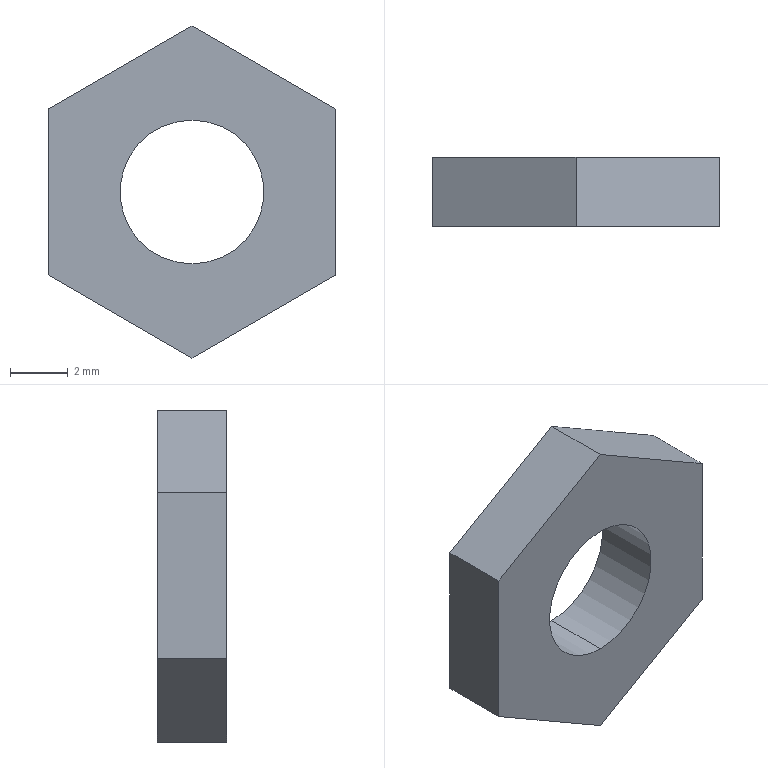Part | SolidWorks | features Extrusion 1, HoleWzd 1 | 1 solid | 10 faces | box 10 x 2.4 x 11.547 mm | volume 160.722 mm3 | plane 8 | cylinder 2 | commonest cylinder face diameters 5 x2
STEP:
#1=CARTESIAN_POINT('',(0.,0.,-2.5));
#2=VERTEX_POINT('',#1);
#3=CARTESIAN_POINT('',(0.,0.,2.5));
#4=VERTEX_POINT('',#3);
#5=CARTESIAN_POINT('',(0.,0.,0.));
#6=DIRECTION('',(0.,1.,0.));
#7=DIRECTION('',(0.,0.,1.));
#8=AXIS2_PLACEMENT_3D('',#5,#6,#7);
#9=CIRCLE('',#8,2.5);
#10=EDGE_CURVE('',#2,#4,#9,.T.);
#11=ORIENTED_EDGE('',*,*,#10,.F.);
#12=CARTESIAN_POINT('',(0.,2.4,-2.5));
#13=VERTEX_POINT('',#12);
#14=CARTESIAN_POINT('',(0.,2.4,-2.5));
#15=DIRECTION('',(0.,1.,0.));
#16=VECTOR('',#15,1000.);
#17=LINE('',#14,#16);
#18=EDGE_CURVE('',#2,#13,#17,.T.);
#19=ORIENTED_EDGE('',*,*,#18,.T.);
#20=CARTESIAN_POINT('',(0.,2.4,2.5));
#21=VERTEX_POINT('',#20);
#22=CARTESIAN_POINT('',(0.,2.4,0.));
#23=DIRECTION('',(0.,1.,0.));
#24=DIRECTION('',(0.,0.,1.));
#25=AXIS2_PLACEMENT_3D('',#22,#23,#24);
#26=CIRCLE('',#25,2.5);
#27=EDGE_CURVE('',#13,#21,#26,.T.);
#28=ORIENTED_EDGE('',*,*,#27,.T.);
#29=CARTESIAN_POINT('',(0.,2.4,2.5));
#30=DIRECTION('',(0.,1.,0.));
#31=VECTOR('',#30,1000.);
#32=LINE('',#29,#31);
#33=EDGE_CURVE('',#4,#21,#32,.T.);
#34=ORIENTED_EDGE('',*,*,#33,.F.);
#35=EDGE_LOOP('',(#11,#19,#28,#34));
#36=FACE_OUTER_BOUND('',#35,.T.);
#37=CARTESIAN_POINT('',(0.,2.4,0.));
#38=DIRECTION('',(0.,1.,0.));
#39=DIRECTION('',(0.,0.,1.));
#40=AXIS2_PLACEMENT_3D('',#37,#38,#39);
#41=CYLINDRICAL_SURFACE('',#40,2.5);
#42=ADVANCED_FACE('',(#36),#41,.F.);
#43=CARTESIAN_POINT('',(5.,0.,-2.887));
#44=VERTEX_POINT('',#43);
#45=CARTESIAN_POINT('',(0.,0.,-5.774));
#46=VERTEX_POINT('',#45);
#47=CARTESIAN_POINT('',(5.,0.,-2.887));
#48=DIRECTION('',(-0.866,0.,-0.5));
#49=VECTOR('',#48,1000.);
#50=LINE('',#47,#49);
#51=EDGE_CURVE('',#44,#46,#50,.T.);
#52=ORIENTED_EDGE('',*,*,#51,.T.);
#53=CARTESIAN_POINT('',(0.,2.4,-5.774));
#54=VERTEX_POINT('',#53);
#55=CARTESIAN_POINT('',(0.,2.4,-5.774));
#56=DIRECTION('',(0.,-1.,0.));
#57=VECTOR('',#56,1000.);
#58=LINE('',#55,#57);
#59=EDGE_CURVE('',#54,#46,#58,.T.);
#60=ORIENTED_EDGE('',*,*,#59,.F.);
#61=CARTESIAN_POINT('',(5.,2.4,-2.887));
#62=VERTEX_POINT('',#61);
#63=CARTESIAN_POINT('',(5.,2.4,-2.887));
#64=DIRECTION('',(-0.866,0.,-0.5));
#65=VECTOR('',#64,1000.);
#66=LINE('',#63,#65);
#67=EDGE_CURVE('',#62,#54,#66,.T.);
#68=ORIENTED_EDGE('',*,*,#67,.F.);
#69=CARTESIAN_POINT('',(5.,2.4,-2.887));
#70=DIRECTION('',(0.,-1.,0.));
#71=VECTOR('',#70,1000.);
#72=LINE('',#69,#71);
#73=EDGE_CURVE('',#62,#44,#72,.T.);
#74=ORIENTED_EDGE('',*,*,#73,.T.);
#75=EDGE_LOOP('',(#52,#60,#68,#74));
#76=FACE_OUTER_BOUND('',#75,.T.);
#77=CARTESIAN_POINT('',(5.,2.4,-2.887));
#78=DIRECTION('',(-0.5,0.,0.866));
#79=DIRECTION('',(0.866,0.,0.5));
#80=AXIS2_PLACEMENT_3D('',#77,#78,#79);
#81=PLANE('',#80);
#82=ADVANCED_FACE('',(#76),#81,.F.);
#83=CARTESIAN_POINT('',(-5.,0.,-2.887));
#84=VERTEX_POINT('',#83);
#85=CARTESIAN_POINT('',(0.,0.,-5.774));
#86=DIRECTION('',(-0.866,0.,0.5));
#87=VECTOR('',#86,1000.);
#88=LINE('',#85,#87);
#89=EDGE_CURVE('',#46,#84,#88,.T.);
#90=ORIENTED_EDGE('',*,*,#89,.T.);
#91=CARTESIAN_POINT('',(-5.,2.4,-2.887));
#92=VERTEX_POINT('',#91);
#93=CARTESIAN_POINT('',(-5.,2.4,-2.887));
#94=DIRECTION('',(0.,-1.,0.));
#95=VECTOR('',#94,1000.);
#96=LINE('',#93,#95);
#97=EDGE_CURVE('',#92,#84,#96,.T.);
#98=ORIENTED_EDGE('',*,*,#97,.F.);
#99=CARTESIAN_POINT('',(0.,2.4,-5.774));
#100=DIRECTION('',(-0.866,0.,0.5));
#101=VECTOR('',#100,1000.);
#102=LINE('',#99,#101);
#103=EDGE_CURVE('',#54,#92,#102,.T.);
#104=ORIENTED_EDGE('',*,*,#103,.F.);
#105=ORIENTED_EDGE('',*,*,#59,.T.);
#106=EDGE_LOOP('',(#90,#98,#104,#105));
#107=FACE_OUTER_BOUND('',#106,.T.);
#108=CARTESIAN_POINT('',(0.,2.4,-5.774));
#109=DIRECTION('',(0.5,0.,0.866));
#110=DIRECTION('',(0.866,0.,-0.5));
#111=AXIS2_PLACEMENT_3D('',#108,#109,#110);
#112=PLANE('',#111);
#113=ADVANCED_FACE('',(#107),#112,.F.);
#114=CARTESIAN_POINT('',(-5.,0.,2.887));
#115=VERTEX_POINT('',#114);
#116=CARTESIAN_POINT('',(-5.,0.,-2.887));
#117=DIRECTION('',(0.,0.,1.));
#118=VECTOR('',#117,1000.);
#119=LINE('',#116,#118);
#120=EDGE_CURVE('',#84,#115,#119,.T.);
#121=ORIENTED_EDGE('',*,*,#120,.T.);
#122=CARTESIAN_POINT('',(-5.,2.4,2.887));
#123=VERTEX_POINT('',#122);
#124=CARTESIAN_POINT('',(-5.,2.4,2.887));
#125=DIRECTION('',(0.,-1.,0.));
#126=VECTOR('',#125,1000.);
#127=LINE('',#124,#126);
#128=EDGE_CURVE('',#123,#115,#127,.T.);
#129=ORIENTED_EDGE('',*,*,#128,.F.);
#130=CARTESIAN_POINT('',(-5.,2.4,-2.887));
#131=DIRECTION('',(0.,0.,1.));
#132=VECTOR('',#131,1000.);
#133=LINE('',#130,#132);
#134=EDGE_CURVE('',#92,#123,#133,.T.);
#135=ORIENTED_EDGE('',*,*,#134,.F.);
#136=ORIENTED_EDGE('',*,*,#97,.T.);
#137=EDGE_LOOP('',(#121,#129,#135,#136));
#138=FACE_OUTER_BOUND('',#137,.T.);
#139=CARTESIAN_POINT('',(-5.,2.4,-2.887));
#140=DIRECTION('',(1.,0.,0.));
#141=DIRECTION('',(0.,0.,-1.));
#142=AXIS2_PLACEMENT_3D('',#139,#140,#141);
#143=PLANE('',#142);
#144=ADVANCED_FACE('',(#138),#143,.F.);
#145=CARTESIAN_POINT('',(0.,0.,5.774));
#146=VERTEX_POINT('',#145);
#147=CARTESIAN_POINT('',(-5.,0.,2.887));
#148=DIRECTION('',(0.866,0.,0.5));
#149=VECTOR('',#148,1000.);
#150=LINE('',#147,#149);
#151=EDGE_CURVE('',#115,#146,#150,.T.);
#152=ORIENTED_EDGE('',*,*,#151,.T.);
#153=CARTESIAN_POINT('',(0.,2.4,5.774));
#154=VERTEX_POINT('',#153);
#155=CARTESIAN_POINT('',(0.,2.4,5.774));
#156=DIRECTION('',(0.,-1.,0.));
#157=VECTOR('',#156,1000.);
#158=LINE('',#155,#157);
#159=EDGE_CURVE('',#154,#146,#158,.T.);
#160=ORIENTED_EDGE('',*,*,#159,.F.);
#161=CARTESIAN_POINT('',(-5.,2.4,2.887));
#162=DIRECTION('',(0.866,0.,0.5));
#163=VECTOR('',#162,1000.);
#164=LINE('',#161,#163);
#165=EDGE_CURVE('',#123,#154,#164,.T.);
#166=ORIENTED_EDGE('',*,*,#165,.F.);
#167=ORIENTED_EDGE('',*,*,#128,.T.);
#168=EDGE_LOOP('',(#152,#160,#166,#167));
#169=FACE_OUTER_BOUND('',#168,.T.);
#170=CARTESIAN_POINT('',(-5.,2.4,2.887));
#171=DIRECTION('',(0.5,0.,-0.866));
#172=DIRECTION('',(-0.866,0.,-0.5));
#173=AXIS2_PLACEMENT_3D('',#170,#171,#172);
#174=PLANE('',#173);
#175=ADVANCED_FACE('',(#169),#174,.F.);
#176=CARTESIAN_POINT('',(5.,0.,2.887));
#177=VERTEX_POINT('',#176);
#178=CARTESIAN_POINT('',(0.,0.,5.774));
#179=DIRECTION('',(0.866,0.,-0.5));
#180=VECTOR('',#179,1000.);
#181=LINE('',#178,#180);
#182=EDGE_CURVE('',#146,#177,#181,.T.);
#183=ORIENTED_EDGE('',*,*,#182,.T.);
#184=CARTESIAN_POINT('',(5.,2.4,2.887));
#185=VERTEX_POINT('',#184);
#186=CARTESIAN_POINT('',(5.,2.4,2.887));
#187=DIRECTION('',(0.,-1.,0.));
#188=VECTOR('',#187,1000.);
#189=LINE('',#186,#188);
#190=EDGE_CURVE('',#185,#177,#189,.T.);
#191=ORIENTED_EDGE('',*,*,#190,.F.);
#192=CARTESIAN_POINT('',(0.,2.4,5.774));
#193=DIRECTION('',(0.866,0.,-0.5));
#194=VECTOR('',#193,1000.);
#195=LINE('',#192,#194);
#196=EDGE_CURVE('',#154,#185,#195,.T.);
#197=ORIENTED_EDGE('',*,*,#196,.F.);
#198=ORIENTED_EDGE('',*,*,#159,.T.);
#199=EDGE_LOOP('',(#183,#191,#197,#198));
#200=FACE_OUTER_BOUND('',#199,.T.);
#201=CARTESIAN_POINT('',(0.,2.4,5.774));
#202=DIRECTION('',(-0.5,0.,-0.866));
#203=DIRECTION('',(-0.866,0.,0.5));
#204=AXIS2_PLACEMENT_3D('',#201,#202,#203);
#205=PLANE('',#204);
#206=ADVANCED_FACE('',(#200),#205,.F.);
#207=CARTESIAN_POINT('',(5.,0.,2.887));
#208=DIRECTION('',(0.,0.,-1.));
#209=VECTOR('',#208,1000.);
#210=LINE('',#207,#209);
#211=EDGE_CURVE('',#177,#44,#210,.T.);
#212=ORIENTED_EDGE('',*,*,#211,.T.);
#213=ORIENTED_EDGE('',*,*,#73,.F.);
#214=CARTESIAN_POINT('',(5.,2.4,2.887));
#215=DIRECTION('',(0.,0.,-1.));
#216=VECTOR('',#215,1000.);
#217=LINE('',#214,#216);
#218=EDGE_CURVE('',#185,#62,#217,.T.);
#219=ORIENTED_EDGE('',*,*,#218,.F.);
#220=ORIENTED_EDGE('',*,*,#190,.T.);
#221=EDGE_LOOP('',(#212,#213,#219,#220));
#222=FACE_OUTER_BOUND('',#221,.T.);
#223=CARTESIAN_POINT('',(5.,2.4,2.887));
#224=DIRECTION('',(-1.,0.,0.));
#225=DIRECTION('',(0.,0.,1.));
#226=AXIS2_PLACEMENT_3D('',#223,#224,#225);
#227=PLANE('',#226);
#228=ADVANCED_FACE('',(#222),#227,.F.);
#229=CARTESIAN_POINT('',(0.,2.4,0.));
#230=DIRECTION('',(0.,1.,0.));
#231=DIRECTION('',(0.,0.,1.));
#232=AXIS2_PLACEMENT_3D('',#229,#230,#231);
#233=CIRCLE('',#232,2.5);
#234=EDGE_CURVE('',#21,#13,#233,.T.);
#235=ORIENTED_EDGE('',*,*,#234,.F.);
#236=ORIENTED_EDGE('',*,*,#27,.F.);
#237=EDGE_LOOP('',(#235,#236));
#238=FACE_BOUND('',#237,.T.);
#239=ORIENTED_EDGE('',*,*,#67,.T.);
#240=ORIENTED_EDGE('',*,*,#103,.T.);
#241=ORIENTED_EDGE('',*,*,#134,.T.);
#242=ORIENTED_EDGE('',*,*,#165,.T.);
#243=ORIENTED_EDGE('',*,*,#196,.T.);
#244=ORIENTED_EDGE('',*,*,#218,.T.);
#245=EDGE_LOOP('',(#239,#240,#241,#242,#243,#244));
#246=FACE_OUTER_BOUND('',#245,.T.);
#247=CARTESIAN_POINT('',(0.,2.4,0.));
#248=DIRECTION('',(0.,1.,0.));
#249=DIRECTION('',(0.,0.,1.));
#250=AXIS2_PLACEMENT_3D('',#247,#248,#249);
#251=PLANE('',#250);
#252=ADVANCED_FACE('',(#238,#246),#251,.T.);
#253=CARTESIAN_POINT('',(0.,0.,0.));
#254=DIRECTION('',(0.,1.,0.));
#255=DIRECTION('',(0.,0.,1.));
#256=AXIS2_PLACEMENT_3D('',#253,#254,#255);
#257=CIRCLE('',#256,2.5);
#258=EDGE_CURVE('',#4,#2,#257,.T.);
#259=ORIENTED_EDGE('',*,*,#258,.T.);
#260=ORIENTED_EDGE('',*,*,#10,.T.);
#261=EDGE_LOOP('',(#259,#260));
#262=FACE_BOUND('',#261,.T.);
#263=ORIENTED_EDGE('',*,*,#51,.F.);
#264=ORIENTED_EDGE('',*,*,#211,.F.);
#265=ORIENTED_EDGE('',*,*,#182,.F.);
#266=ORIENTED_EDGE('',*,*,#151,.F.);
#267=ORIENTED_EDGE('',*,*,#120,.F.);
#268=ORIENTED_EDGE('',*,*,#89,.F.);
#269=EDGE_LOOP('',(#263,#264,#265,#266,#267,#268));
#270=FACE_OUTER_BOUND('',#269,.T.);
#271=CARTESIAN_POINT('',(0.,0.,0.));
#272=DIRECTION('',(0.,1.,0.));
#273=DIRECTION('',(0.,0.,1.));
#274=AXIS2_PLACEMENT_3D('',#271,#272,#273);
#275=PLANE('',#274);
#276=ADVANCED_FACE('',(#262,#270),#275,.F.);
#277=ORIENTED_EDGE('',*,*,#18,.F.);
#278=ORIENTED_EDGE('',*,*,#258,.F.);
#279=ORIENTED_EDGE('',*,*,#33,.T.);
#280=ORIENTED_EDGE('',*,*,#234,.T.);
#281=EDGE_LOOP('',(#277,#278,#279,#280));
#282=FACE_OUTER_BOUND('',#281,.T.);
#283=CARTESIAN_POINT('',(0.,2.4,0.));
#284=DIRECTION('',(0.,1.,0.));
#285=DIRECTION('',(0.,0.,1.));
#286=AXIS2_PLACEMENT_3D('',#283,#284,#285);
#287=CYLINDRICAL_SURFACE('',#286,2.5);
#288=ADVANCED_FACE('',(#282),#287,.F.);
#289=CLOSED_SHELL('',(#42,#82,#113,#144,#175,#206,#228,#252,#276,#288));
#290=MANIFOLD_SOLID_BREP('',#289);
#291=CARTESIAN_POINT('',(0.,0.,0.));
#292=DIRECTION('',(0.,0.,1.));
#293=DIRECTION('',(1.,0.,0.));
#294=AXIS2_PLACEMENT_3D('',#291,#292,#293);
#295=(LENGTH_UNIT()NAMED_UNIT(*)SI_UNIT(.MILLI.,.METRE.));
#296=UNCERTAINTY_MEASURE_WITH_UNIT(LENGTH_MEASURE(0.00001),#295,'','');
#297=(NAMED_UNIT(*)PLANE_ANGLE_UNIT()SI_UNIT($,.RADIAN.));
#298=(NAMED_UNIT(*)SI_UNIT($,.STERADIAN.)SOLID_ANGLE_UNIT());
#299=(GEOMETRIC_REPRESENTATION_CONTEXT(3)GLOBAL_UNCERTAINTY_ASSIGNED_CONTEXT((#296))GLOBAL_UNIT_ASSIGNED_CONTEXT((#295,#297,#298))REPRESENTATION_CONTEXT('',''));
#300=ADVANCED_BREP_SHAPE_REPRESENTATION('',(#290,#294),#299);